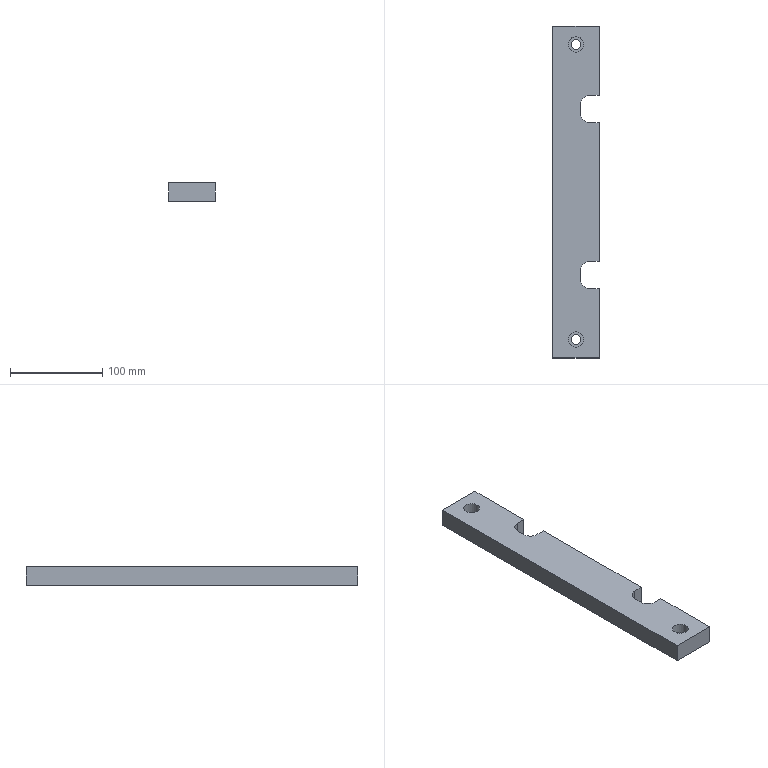Part | STEP file | 200 mesh_id2002 | 1 solid | 24 faces | box 50 x 360 x 20 mm | volume 331105 mm3 | plane 16 | cylinder 8 | commonest cylinder face diameters 20 x4 10.7 x2 17 x2
STEP:
#1=CARTESIAN_POINT('',(-17103.234,-4180.269,185.258));
#2=VERTEX_POINT('',#1);
#3=CARTESIAN_POINT('',(-17097.884,-4180.269,185.258));
#4=DIRECTION('',(0.,0.,1.));
#5=DIRECTION('',(-1.,0.,0.));
#6=AXIS2_PLACEMENT_3D('',#3,#4,#5);
#7=CIRCLE('',#6,5.35);
#8=EDGE_CURVE('',#2,#2,#7,.T.);
#9=ORIENTED_EDGE('',*,*,#8,.F.);
#10=EDGE_LOOP('',(#9));
#11=FACE_BOUND('',#10,.T.);
#12=CARTESIAN_POINT('',(-17106.384,-4180.269,185.258));
#13=VERTEX_POINT('',#12);
#14=CARTESIAN_POINT('',(-17097.884,-4180.269,185.258));
#15=DIRECTION('',(0.,0.,1.));
#16=DIRECTION('',(-1.,0.,0.));
#17=AXIS2_PLACEMENT_3D('',#14,#15,#16);
#18=CIRCLE('',#17,8.5);
#19=EDGE_CURVE('',#13,#13,#18,.T.);
#20=ORIENTED_EDGE('',*,*,#19,.T.);
#21=EDGE_LOOP('',(#20));
#22=FACE_BOUND('',#21,.T.);
#23=CARTESIAN_POINT('',(-17097.884,-4180.269,185.258));
#24=DIRECTION('',(0.,0.,-1.));
#25=DIRECTION('',(-1.,0.,0.));
#26=AXIS2_PLACEMENT_3D('',#23,#24,#25);
#27=PLANE('',#26);
#28=ADVANCED_FACE('',(#11,#22),#27,.F.);
#29=ORIENTED_EDGE('',*,*,#19,.F.);
#30=EDGE_LOOP('',(#29));
#31=FACE_BOUND('',#30,.T.);
#32=CARTESIAN_POINT('',(-17106.384,-4180.269,196.258));
#33=VERTEX_POINT('',#32);
#34=CARTESIAN_POINT('',(-17097.884,-4180.269,196.258));
#35=DIRECTION('',(0.,0.,-1.));
#36=DIRECTION('',(-1.,0.,0.));
#37=AXIS2_PLACEMENT_3D('',#34,#35,#36);
#38=CIRCLE('',#37,8.5);
#39=EDGE_CURVE('',#33,#33,#38,.T.);
#40=ORIENTED_EDGE('',*,*,#39,.F.);
#41=EDGE_LOOP('',(#40));
#42=FACE_BOUND('',#41,.T.);
#43=CARTESIAN_POINT('',(-17097.884,-4180.269,196.258));
#44=DIRECTION('',(0.,0.,-1.));
#45=DIRECTION('',(-1.,0.,0.));
#46=AXIS2_PLACEMENT_3D('',#43,#44,#45);
#47=CYLINDRICAL_SURFACE('',#46,8.5);
#48=ADVANCED_FACE('',(#31,#42),#47,.F.);
#49=ORIENTED_EDGE('',*,*,#8,.T.);
#50=EDGE_LOOP('',(#49));
#51=FACE_BOUND('',#50,.T.);
#52=CARTESIAN_POINT('',(-17092.534,-4180.269,176.258));
#53=VERTEX_POINT('',#52);
#54=CARTESIAN_POINT('',(-17097.884,-4180.269,176.258));
#55=DIRECTION('',(0.,0.,1.));
#56=DIRECTION('',(1.,0.,0.));
#57=AXIS2_PLACEMENT_3D('',#54,#55,#56);
#58=CIRCLE('',#57,5.35);
#59=EDGE_CURVE('',#53,#53,#58,.T.);
#60=ORIENTED_EDGE('',*,*,#59,.F.);
#61=EDGE_LOOP('',(#60));
#62=FACE_BOUND('',#61,.T.);
#63=CARTESIAN_POINT('',(-17097.884,-4180.269,65.92));
#64=DIRECTION('',(0.,0.,-1.));
#65=DIRECTION('',(-1.,0.,0.));
#66=AXIS2_PLACEMENT_3D('',#63,#64,#65);
#67=CYLINDRICAL_SURFACE('',#66,5.35);
#68=ADVANCED_FACE('',(#51,#62),#67,.F.);
#69=CARTESIAN_POINT('',(-17103.234,-3860.269,185.258));
#70=VERTEX_POINT('',#69);
#71=CARTESIAN_POINT('',(-17097.884,-3860.269,185.258));
#72=DIRECTION('',(0.,0.,1.));
#73=DIRECTION('',(-1.,0.,0.));
#74=AXIS2_PLACEMENT_3D('',#71,#72,#73);
#75=CIRCLE('',#74,5.35);
#76=EDGE_CURVE('',#70,#70,#75,.T.);
#77=ORIENTED_EDGE('',*,*,#76,.F.);
#78=EDGE_LOOP('',(#77));
#79=FACE_BOUND('',#78,.T.);
#80=CARTESIAN_POINT('',(-17106.384,-3860.269,185.258));
#81=VERTEX_POINT('',#80);
#82=CARTESIAN_POINT('',(-17097.884,-3860.269,185.258));
#83=DIRECTION('',(0.,0.,1.));
#84=DIRECTION('',(-1.,0.,0.));
#85=AXIS2_PLACEMENT_3D('',#82,#83,#84);
#86=CIRCLE('',#85,8.5);
#87=EDGE_CURVE('',#81,#81,#86,.T.);
#88=ORIENTED_EDGE('',*,*,#87,.T.);
#89=EDGE_LOOP('',(#88));
#90=FACE_BOUND('',#89,.T.);
#91=CARTESIAN_POINT('',(-17097.884,-3860.269,185.258));
#92=DIRECTION('',(0.,0.,-1.));
#93=DIRECTION('',(-1.,0.,0.));
#94=AXIS2_PLACEMENT_3D('',#91,#92,#93);
#95=PLANE('',#94);
#96=ADVANCED_FACE('',(#79,#90),#95,.F.);
#97=CARTESIAN_POINT('',(-17082.884,-3945.269,196.258));
#98=VERTEX_POINT('',#97);
#99=CARTESIAN_POINT('',(-17092.884,-3935.269,196.258));
#100=VERTEX_POINT('',#99);
#101=CARTESIAN_POINT('',(-17082.884,-3935.269,196.258));
#102=DIRECTION('',(0.,0.,-1.));
#103=DIRECTION('',(-1.,0.,0.));
#104=AXIS2_PLACEMENT_3D('',#101,#102,#103);
#105=CIRCLE('',#104,10.);
#106=EDGE_CURVE('',#98,#100,#105,.T.);
#107=ORIENTED_EDGE('',*,*,#106,.F.);
#108=CARTESIAN_POINT('',(-17082.884,-3945.269,176.258));
#109=VERTEX_POINT('',#108);
#110=CARTESIAN_POINT('',(-17082.884,-3945.269,196.258));
#111=DIRECTION('',(0.,0.,1.));
#112=VECTOR('',#111,1.);
#113=LINE('',#110,#112);
#114=EDGE_CURVE('',#109,#98,#113,.T.);
#115=ORIENTED_EDGE('',*,*,#114,.F.);
#116=CARTESIAN_POINT('',(-17092.884,-3935.269,176.258));
#117=VERTEX_POINT('',#116);
#118=CARTESIAN_POINT('',(-17082.884,-3935.269,176.258));
#119=DIRECTION('',(0.,0.,1.));
#120=DIRECTION('',(1.,0.,0.));
#121=AXIS2_PLACEMENT_3D('',#118,#119,#120);
#122=CIRCLE('',#121,10.);
#123=EDGE_CURVE('',#117,#109,#122,.T.);
#124=ORIENTED_EDGE('',*,*,#123,.F.);
#125=CARTESIAN_POINT('',(-17092.884,-3935.269,176.258));
#126=DIRECTION('',(0.,0.,-1.));
#127=VECTOR('',#126,1.);
#128=LINE('',#125,#127);
#129=EDGE_CURVE('',#100,#117,#128,.T.);
#130=ORIENTED_EDGE('',*,*,#129,.F.);
#131=EDGE_LOOP('',(#107,#115,#124,#130));
#132=FACE_OUTER_BOUND('',#131,.T.);
#133=CARTESIAN_POINT('',(-17082.884,-3935.269,176.258));
#134=DIRECTION('',(0.,0.,1.));
#135=DIRECTION('',(1.,0.,0.));
#136=AXIS2_PLACEMENT_3D('',#133,#134,#135);
#137=CYLINDRICAL_SURFACE('',#136,10.);
#138=ADVANCED_FACE('',(#132),#137,.F.);
#139=CARTESIAN_POINT('',(-17072.884,-3945.269,176.258));
#140=VERTEX_POINT('',#139);
#141=CARTESIAN_POINT('',(-17082.884,-3945.269,176.258));
#142=DIRECTION('',(1.,0.,0.));
#143=VECTOR('',#142,1.);
#144=LINE('',#141,#143);
#145=EDGE_CURVE('',#109,#140,#144,.T.);
#146=ORIENTED_EDGE('',*,*,#145,.F.);
#147=ORIENTED_EDGE('',*,*,#114,.T.);
#148=CARTESIAN_POINT('',(-17072.884,-3945.269,196.258));
#149=VERTEX_POINT('',#148);
#150=CARTESIAN_POINT('',(-17082.884,-3945.269,196.258));
#151=DIRECTION('',(-1.,0.,0.));
#152=VECTOR('',#151,1.);
#153=LINE('',#150,#152);
#154=EDGE_CURVE('',#149,#98,#153,.T.);
#155=ORIENTED_EDGE('',*,*,#154,.F.);
#156=CARTESIAN_POINT('',(-17072.884,-3945.269,176.258));
#157=DIRECTION('',(0.,0.,1.));
#158=VECTOR('',#157,1.);
#159=LINE('',#156,#158);
#160=EDGE_CURVE('',#140,#149,#159,.T.);
#161=ORIENTED_EDGE('',*,*,#160,.F.);
#162=EDGE_LOOP('',(#146,#147,#155,#161));
#163=FACE_OUTER_BOUND('',#162,.T.);
#164=CARTESIAN_POINT('',(-17082.884,-3945.269,176.258));
#165=DIRECTION('',(0.,-1.,0.));
#166=DIRECTION('',(0.,0.,-1.));
#167=AXIS2_PLACEMENT_3D('',#164,#165,#166);
#168=PLANE('',#167);
#169=ADVANCED_FACE('',(#163),#168,.F.);
#170=CARTESIAN_POINT('',(-17072.884,-4095.269,176.258));
#171=VERTEX_POINT('',#170);
#172=CARTESIAN_POINT('',(-17072.884,-3830.269,176.258));
#173=DIRECTION('',(0.,-1.,0.));
#174=VECTOR('',#173,1.);
#175=LINE('',#172,#174);
#176=EDGE_CURVE('',#140,#171,#175,.T.);
#177=ORIENTED_EDGE('',*,*,#176,.F.);
#178=ORIENTED_EDGE('',*,*,#160,.T.);
#179=CARTESIAN_POINT('',(-17072.884,-4095.269,196.258));
#180=VERTEX_POINT('',#179);
#181=CARTESIAN_POINT('',(-17072.884,-4210.269,196.258));
#182=DIRECTION('',(0.,1.,0.));
#183=VECTOR('',#182,1.);
#184=LINE('',#181,#183);
#185=EDGE_CURVE('',#180,#149,#184,.T.);
#186=ORIENTED_EDGE('',*,*,#185,.F.);
#187=CARTESIAN_POINT('',(-17072.884,-4095.269,176.258));
#188=DIRECTION('',(0.,0.,1.));
#189=VECTOR('',#188,1.);
#190=LINE('',#187,#189);
#191=EDGE_CURVE('',#171,#180,#190,.T.);
#192=ORIENTED_EDGE('',*,*,#191,.F.);
#193=EDGE_LOOP('',(#177,#178,#186,#192));
#194=FACE_OUTER_BOUND('',#193,.T.);
#195=CARTESIAN_POINT('',(-17072.884,0.,15.));
#196=DIRECTION('',(-1.,0.,0.));
#197=DIRECTION('',(0.,0.,1.));
#198=AXIS2_PLACEMENT_3D('',#195,#196,#197);
#199=PLANE('',#198);
#200=ADVANCED_FACE('',(#194),#199,.F.);
#201=CARTESIAN_POINT('',(-17082.884,-4095.269,196.258));
#202=VERTEX_POINT('',#201);
#203=CARTESIAN_POINT('',(-17082.884,-4095.269,196.258));
#204=DIRECTION('',(1.,0.,0.));
#205=VECTOR('',#204,1.);
#206=LINE('',#203,#205);
#207=EDGE_CURVE('',#202,#180,#206,.T.);
#208=ORIENTED_EDGE('',*,*,#207,.F.);
#209=CARTESIAN_POINT('',(-17082.884,-4095.269,176.258));
#210=VERTEX_POINT('',#209);
#211=CARTESIAN_POINT('',(-17082.884,-4095.269,176.258));
#212=DIRECTION('',(0.,0.,-1.));
#213=VECTOR('',#212,1.);
#214=LINE('',#211,#213);
#215=EDGE_CURVE('',#202,#210,#214,.T.);
#216=ORIENTED_EDGE('',*,*,#215,.T.);
#217=CARTESIAN_POINT('',(-17082.884,-4095.269,176.258));
#218=DIRECTION('',(-1.,0.,0.));
#219=VECTOR('',#218,1.);
#220=LINE('',#217,#219);
#221=EDGE_CURVE('',#171,#210,#220,.T.);
#222=ORIENTED_EDGE('',*,*,#221,.F.);
#223=ORIENTED_EDGE('',*,*,#191,.T.);
#224=EDGE_LOOP('',(#208,#216,#222,#223));
#225=FACE_OUTER_BOUND('',#224,.T.);
#226=CARTESIAN_POINT('',(-17082.884,-4095.269,176.258));
#227=DIRECTION('',(0.,1.,0.));
#228=DIRECTION('',(0.,0.,1.));
#229=AXIS2_PLACEMENT_3D('',#226,#227,#228);
#230=PLANE('',#229);
#231=ADVANCED_FACE('',(#225),#230,.F.);
#232=CARTESIAN_POINT('',(-17092.884,-4105.269,196.258));
#233=VERTEX_POINT('',#232);
#234=CARTESIAN_POINT('',(-17082.884,-4105.269,196.258));
#235=DIRECTION('',(0.,0.,-1.));
#236=DIRECTION('',(-1.,0.,0.));
#237=AXIS2_PLACEMENT_3D('',#234,#235,#236);
#238=CIRCLE('',#237,10.);
#239=EDGE_CURVE('',#233,#202,#238,.T.);
#240=ORIENTED_EDGE('',*,*,#239,.F.);
#241=CARTESIAN_POINT('',(-17092.884,-4105.269,176.258));
#242=VERTEX_POINT('',#241);
#243=CARTESIAN_POINT('',(-17092.884,-4105.269,196.258));
#244=DIRECTION('',(0.,0.,1.));
#245=VECTOR('',#244,1.);
#246=LINE('',#243,#245);
#247=EDGE_CURVE('',#242,#233,#246,.T.);
#248=ORIENTED_EDGE('',*,*,#247,.F.);
#249=CARTESIAN_POINT('',(-17082.884,-4105.269,176.258));
#250=DIRECTION('',(0.,0.,1.));
#251=DIRECTION('',(1.,0.,0.));
#252=AXIS2_PLACEMENT_3D('',#249,#250,#251);
#253=CIRCLE('',#252,10.);
#254=EDGE_CURVE('',#210,#242,#253,.T.);
#255=ORIENTED_EDGE('',*,*,#254,.F.);
#256=ORIENTED_EDGE('',*,*,#215,.F.);
#257=EDGE_LOOP('',(#240,#248,#255,#256));
#258=FACE_OUTER_BOUND('',#257,.T.);
#259=CARTESIAN_POINT('',(-17082.884,-4105.269,176.258));
#260=DIRECTION('',(0.,0.,1.));
#261=DIRECTION('',(1.,0.,0.));
#262=AXIS2_PLACEMENT_3D('',#259,#260,#261);
#263=CYLINDRICAL_SURFACE('',#262,10.);
#264=ADVANCED_FACE('',(#258),#263,.F.);
#265=CARTESIAN_POINT('',(-17092.884,-4115.269,196.258));
#266=VERTEX_POINT('',#265);
#267=CARTESIAN_POINT('',(-17092.884,-4110.269,196.258));
#268=DIRECTION('',(0.,1.,0.));
#269=VECTOR('',#268,1.);
#270=LINE('',#267,#269);
#271=EDGE_CURVE('',#266,#233,#270,.T.);
#272=ORIENTED_EDGE('',*,*,#271,.F.);
#273=CARTESIAN_POINT('',(-17092.884,-4115.269,176.258));
#274=VERTEX_POINT('',#273);
#275=CARTESIAN_POINT('',(-17092.884,-4115.269,176.258));
#276=DIRECTION('',(0.,0.,-1.));
#277=VECTOR('',#276,1.);
#278=LINE('',#275,#277);
#279=EDGE_CURVE('',#266,#274,#278,.T.);
#280=ORIENTED_EDGE('',*,*,#279,.T.);
#281=CARTESIAN_POINT('',(-17092.884,-4110.269,176.258));
#282=DIRECTION('',(0.,-1.,0.));
#283=VECTOR('',#282,1.);
#284=LINE('',#281,#283);
#285=EDGE_CURVE('',#242,#274,#284,.T.);
#286=ORIENTED_EDGE('',*,*,#285,.F.);
#287=ORIENTED_EDGE('',*,*,#247,.T.);
#288=EDGE_LOOP('',(#272,#280,#286,#287));
#289=FACE_OUTER_BOUND('',#288,.T.);
#290=CARTESIAN_POINT('',(-17092.884,-4110.269,176.258));
#291=DIRECTION('',(-1.,0.,0.));
#292=DIRECTION('',(0.,0.,1.));
#293=AXIS2_PLACEMENT_3D('',#290,#291,#292);
#294=PLANE('',#293);
#295=ADVANCED_FACE('',(#289),#294,.F.);
#296=CARTESIAN_POINT('',(-17082.884,-4125.269,196.258));
#297=VERTEX_POINT('',#296);
#298=CARTESIAN_POINT('',(-17082.884,-4115.269,196.258));
#299=DIRECTION('',(0.,0.,-1.));
#300=DIRECTION('',(-1.,0.,0.));
#301=AXIS2_PLACEMENT_3D('',#298,#299,#300);
#302=CIRCLE('',#301,10.);
#303=EDGE_CURVE('',#297,#266,#302,.T.);
#304=ORIENTED_EDGE('',*,*,#303,.F.);
#305=CARTESIAN_POINT('',(-17082.884,-4125.269,176.258));
#306=VERTEX_POINT('',#305);
#307=CARTESIAN_POINT('',(-17082.884,-4125.269,196.258));
#308=DIRECTION('',(0.,0.,1.));
#309=VECTOR('',#308,1.);
#310=LINE('',#307,#309);
#311=EDGE_CURVE('',#306,#297,#310,.T.);
#312=ORIENTED_EDGE('',*,*,#311,.F.);
#313=CARTESIAN_POINT('',(-17082.884,-4115.269,176.258));
#314=DIRECTION('',(0.,0.,1.));
#315=DIRECTION('',(1.,0.,0.));
#316=AXIS2_PLACEMENT_3D('',#313,#314,#315);
#317=CIRCLE('',#316,10.);
#318=EDGE_CURVE('',#274,#306,#317,.T.);
#319=ORIENTED_EDGE('',*,*,#318,.F.);
#320=ORIENTED_EDGE('',*,*,#279,.F.);
#321=EDGE_LOOP('',(#304,#312,#319,#320));
#322=FACE_OUTER_BOUND('',#321,.T.);
#323=CARTESIAN_POINT('',(-17082.884,-4115.269,176.258));
#324=DIRECTION('',(0.,0.,1.));
#325=DIRECTION('',(1.,0.,0.));
#326=AXIS2_PLACEMENT_3D('',#323,#324,#325);
#327=CYLINDRICAL_SURFACE('',#326,10.);
#328=ADVANCED_FACE('',(#322),#327,.F.);
#329=CARTESIAN_POINT('',(-17072.884,-4125.269,176.258));
#330=VERTEX_POINT('',#329);
#331=CARTESIAN_POINT('',(-17082.884,-4125.269,176.258));
#332=DIRECTION('',(1.,0.,0.));
#333=VECTOR('',#332,1.);
#334=LINE('',#331,#333);
#335=EDGE_CURVE('',#306,#330,#334,.T.);
#336=ORIENTED_EDGE('',*,*,#335,.F.);
#337=ORIENTED_EDGE('',*,*,#311,.T.);
#338=CARTESIAN_POINT('',(-17072.884,-4125.269,196.258));
#339=VERTEX_POINT('',#338);
#340=CARTESIAN_POINT('',(-17082.884,-4125.269,196.258));
#341=DIRECTION('',(-1.,0.,0.));
#342=VECTOR('',#341,1.);
#343=LINE('',#340,#342);
#344=EDGE_CURVE('',#339,#297,#343,.T.);
#345=ORIENTED_EDGE('',*,*,#344,.F.);
#346=CARTESIAN_POINT('',(-17072.884,-4125.269,176.258));
#347=DIRECTION('',(0.,0.,1.));
#348=VECTOR('',#347,1.);
#349=LINE('',#346,#348);
#350=EDGE_CURVE('',#330,#339,#349,.T.);
#351=ORIENTED_EDGE('',*,*,#350,.F.);
#352=EDGE_LOOP('',(#336,#337,#345,#351));
#353=FACE_OUTER_BOUND('',#352,.T.);
#354=CARTESIAN_POINT('',(-17082.884,-4125.269,176.258));
#355=DIRECTION('',(0.,-1.,0.));
#356=DIRECTION('',(0.,0.,-1.));
#357=AXIS2_PLACEMENT_3D('',#354,#355,#356);
#358=PLANE('',#357);
#359=ADVANCED_FACE('',(#353),#358,.F.);
#360=CARTESIAN_POINT('',(-17072.884,-4200.269,176.258));
#361=VERTEX_POINT('',#360);
#362=CARTESIAN_POINT('',(-17072.884,-3830.269,176.258));
#363=DIRECTION('',(0.,-1.,0.));
#364=VECTOR('',#363,1.);
#365=LINE('',#362,#364);
#366=EDGE_CURVE('',#330,#361,#365,.T.);
#367=ORIENTED_EDGE('',*,*,#366,.F.);
#368=ORIENTED_EDGE('',*,*,#350,.T.);
#369=CARTESIAN_POINT('',(-17072.884,-4200.269,196.258));
#370=VERTEX_POINT('',#369);
#371=CARTESIAN_POINT('',(-17072.884,-4210.269,196.258));
#372=DIRECTION('',(0.,1.,0.));
#373=VECTOR('',#372,1.);
#374=LINE('',#371,#373);
#375=EDGE_CURVE('',#370,#339,#374,.T.);
#376=ORIENTED_EDGE('',*,*,#375,.F.);
#377=CARTESIAN_POINT('',(-17072.884,-4200.269,176.258));
#378=DIRECTION('',(0.,0.,1.));
#379=VECTOR('',#378,1.);
#380=LINE('',#377,#379);
#381=EDGE_CURVE('',#361,#370,#380,.T.);
#382=ORIENTED_EDGE('',*,*,#381,.F.);
#383=EDGE_LOOP('',(#367,#368,#376,#382));
#384=FACE_OUTER_BOUND('',#383,.T.);
#385=CARTESIAN_POINT('',(-17072.884,0.,15.));
#386=DIRECTION('',(-1.,0.,0.));
#387=DIRECTION('',(0.,0.,1.));
#388=AXIS2_PLACEMENT_3D('',#385,#386,#387);
#389=PLANE('',#388);
#390=ADVANCED_FACE('',(#384),#389,.F.);
#391=ORIENTED_EDGE('',*,*,#381,.T.);
#392=CARTESIAN_POINT('',(-17122.884,-4200.269,196.258));
#393=VERTEX_POINT('',#392);
#394=CARTESIAN_POINT('',(-17132.884,-4200.269,196.258));
#395=DIRECTION('',(1.,0.,0.));
#396=VECTOR('',#395,1.);
#397=LINE('',#394,#396);
#398=EDGE_CURVE('',#393,#370,#397,.T.);
#399=ORIENTED_EDGE('',*,*,#398,.F.);
#400=CARTESIAN_POINT('',(-17122.884,-4200.269,176.258));
#401=VERTEX_POINT('',#400);
#402=CARTESIAN_POINT('',(-17122.884,-4200.269,176.258));
#403=DIRECTION('',(0.,0.,1.));
#404=VECTOR('',#403,1.);
#405=LINE('',#402,#404);
#406=EDGE_CURVE('',#401,#393,#405,.T.);
#407=ORIENTED_EDGE('',*,*,#406,.F.);
#408=CARTESIAN_POINT('',(-17132.884,-4200.269,176.258));
#409=DIRECTION('',(1.,0.,0.));
#410=VECTOR('',#409,1.);
#411=LINE('',#408,#410);
#412=EDGE_CURVE('',#401,#361,#411,.T.);
#413=ORIENTED_EDGE('',*,*,#412,.T.);
#414=EDGE_LOOP('',(#391,#399,#407,#413));
#415=FACE_OUTER_BOUND('',#414,.T.);
#416=CARTESIAN_POINT('',(-17132.884,-4200.269,176.258));
#417=DIRECTION('',(0.,1.,0.));
#418=DIRECTION('',(0.,0.,1.));
#419=AXIS2_PLACEMENT_3D('',#416,#417,#418);
#420=PLANE('',#419);
#421=ADVANCED_FACE('',(#415),#420,.F.);
#422=ORIENTED_EDGE('',*,*,#406,.T.);
#423=CARTESIAN_POINT('',(-17122.884,-3840.269,196.258));
#424=VERTEX_POINT('',#423);
#425=CARTESIAN_POINT('',(-17122.884,-4210.269,196.258));
#426=DIRECTION('',(0.,1.,0.));
#427=VECTOR('',#426,1.);
#428=LINE('',#425,#427);
#429=EDGE_CURVE('',#393,#424,#428,.T.);
#430=ORIENTED_EDGE('',*,*,#429,.T.);
#431=CARTESIAN_POINT('',(-17122.884,-3840.269,176.258));
#432=VERTEX_POINT('',#431);
#433=CARTESIAN_POINT('',(-17122.884,-3840.269,196.258));
#434=DIRECTION('',(0.,0.,-1.));
#435=VECTOR('',#434,1.);
#436=LINE('',#433,#435);
#437=EDGE_CURVE('',#424,#432,#436,.T.);
#438=ORIENTED_EDGE('',*,*,#437,.T.);
#439=CARTESIAN_POINT('',(-17122.884,-3830.269,176.258));
#440=DIRECTION('',(0.,-1.,0.));
#441=VECTOR('',#440,1.);
#442=LINE('',#439,#441);
#443=EDGE_CURVE('',#432,#401,#442,.T.);
#444=ORIENTED_EDGE('',*,*,#443,.T.);
#445=EDGE_LOOP('',(#422,#430,#438,#444));
#446=FACE_OUTER_BOUND('',#445,.T.);
#447=CARTESIAN_POINT('',(-17122.884,-4180.269,126.258));
#448=DIRECTION('',(1.,0.,0.));
#449=DIRECTION('',(0.,0.,-1.));
#450=AXIS2_PLACEMENT_3D('',#447,#448,#449);
#451=PLANE('',#450);
#452=ADVANCED_FACE('',(#446),#451,.F.);
#453=CARTESIAN_POINT('',(-17072.884,-3840.269,196.258));
#454=VERTEX_POINT('',#453);
#455=CARTESIAN_POINT('',(-17072.884,-3840.269,176.258));
#456=VERTEX_POINT('',#455);
#457=CARTESIAN_POINT('',(-17072.884,-3840.269,196.258));
#458=DIRECTION('',(0.,0.,-1.));
#459=VECTOR('',#458,1.);
#460=LINE('',#457,#459);
#461=EDGE_CURVE('',#454,#456,#460,.T.);
#462=ORIENTED_EDGE('',*,*,#461,.T.);
#463=CARTESIAN_POINT('',(-17132.884,-3840.269,176.258));
#464=DIRECTION('',(1.,0.,0.));
#465=VECTOR('',#464,1.);
#466=LINE('',#463,#465);
#467=EDGE_CURVE('',#432,#456,#466,.T.);
#468=ORIENTED_EDGE('',*,*,#467,.F.);
#469=ORIENTED_EDGE('',*,*,#437,.F.);
#470=CARTESIAN_POINT('',(-17132.884,-3840.269,196.258));
#471=DIRECTION('',(1.,0.,0.));
#472=VECTOR('',#471,1.);
#473=LINE('',#470,#472);
#474=EDGE_CURVE('',#424,#454,#473,.T.);
#475=ORIENTED_EDGE('',*,*,#474,.T.);
#476=EDGE_LOOP('',(#462,#468,#469,#475));
#477=FACE_OUTER_BOUND('',#476,.T.);
#478=CARTESIAN_POINT('',(-17132.884,-3840.269,196.258));
#479=DIRECTION('',(0.,-1.,0.));
#480=DIRECTION('',(0.,0.,-1.));
#481=AXIS2_PLACEMENT_3D('',#478,#479,#480);
#482=PLANE('',#481);
#483=ADVANCED_FACE('',(#477),#482,.F.);
#484=CARTESIAN_POINT('',(-17072.884,-3915.269,176.258));
#485=VERTEX_POINT('',#484);
#486=CARTESIAN_POINT('',(-17072.884,-3915.269,196.258));
#487=VERTEX_POINT('',#486);
#488=CARTESIAN_POINT('',(-17072.884,-3915.269,176.258));
#489=DIRECTION('',(0.,0.,1.));
#490=VECTOR('',#489,1.);
#491=LINE('',#488,#490);
#492=EDGE_CURVE('',#485,#487,#491,.T.);
#493=ORIENTED_EDGE('',*,*,#492,.F.);
#494=CARTESIAN_POINT('',(-17072.884,-3830.269,176.258));
#495=DIRECTION('',(0.,-1.,0.));
#496=VECTOR('',#495,1.);
#497=LINE('',#494,#496);
#498=EDGE_CURVE('',#456,#485,#497,.T.);
#499=ORIENTED_EDGE('',*,*,#498,.F.);
#500=ORIENTED_EDGE('',*,*,#461,.F.);
#501=CARTESIAN_POINT('',(-17072.884,-4210.269,196.258));
#502=DIRECTION('',(0.,1.,0.));
#503=VECTOR('',#502,1.);
#504=LINE('',#501,#503);
#505=EDGE_CURVE('',#487,#454,#504,.T.);
#506=ORIENTED_EDGE('',*,*,#505,.F.);
#507=EDGE_LOOP('',(#493,#499,#500,#506));
#508=FACE_OUTER_BOUND('',#507,.T.);
#509=CARTESIAN_POINT('',(-17072.884,0.,15.));
#510=DIRECTION('',(-1.,0.,0.));
#511=DIRECTION('',(0.,0.,1.));
#512=AXIS2_PLACEMENT_3D('',#509,#510,#511);
#513=PLANE('',#512);
#514=ADVANCED_FACE('',(#508),#513,.F.);
#515=CARTESIAN_POINT('',(-17082.884,-3915.269,196.258));
#516=VERTEX_POINT('',#515);
#517=CARTESIAN_POINT('',(-17082.884,-3915.269,196.258));
#518=DIRECTION('',(1.,0.,0.));
#519=VECTOR('',#518,1.);
#520=LINE('',#517,#519);
#521=EDGE_CURVE('',#516,#487,#520,.T.);
#522=ORIENTED_EDGE('',*,*,#521,.F.);
#523=CARTESIAN_POINT('',(-17082.884,-3915.269,176.258));
#524=VERTEX_POINT('',#523);
#525=CARTESIAN_POINT('',(-17082.884,-3915.269,176.258));
#526=DIRECTION('',(0.,0.,-1.));
#527=VECTOR('',#526,1.);
#528=LINE('',#525,#527);
#529=EDGE_CURVE('',#516,#524,#528,.T.);
#530=ORIENTED_EDGE('',*,*,#529,.T.);
#531=CARTESIAN_POINT('',(-17082.884,-3915.269,176.258));
#532=DIRECTION('',(-1.,0.,0.));
#533=VECTOR('',#532,1.);
#534=LINE('',#531,#533);
#535=EDGE_CURVE('',#485,#524,#534,.T.);
#536=ORIENTED_EDGE('',*,*,#535,.F.);
#537=ORIENTED_EDGE('',*,*,#492,.T.);
#538=EDGE_LOOP('',(#522,#530,#536,#537));
#539=FACE_OUTER_BOUND('',#538,.T.);
#540=CARTESIAN_POINT('',(-17082.884,-3915.269,176.258));
#541=DIRECTION('',(0.,1.,0.));
#542=DIRECTION('',(0.,0.,1.));
#543=AXIS2_PLACEMENT_3D('',#540,#541,#542);
#544=PLANE('',#543);
#545=ADVANCED_FACE('',(#539),#544,.F.);
#546=CARTESIAN_POINT('',(-17092.884,-3925.269,196.258));
#547=VERTEX_POINT('',#546);
#548=CARTESIAN_POINT('',(-17082.884,-3925.269,196.258));
#549=DIRECTION('',(0.,0.,-1.));
#550=DIRECTION('',(-1.,0.,0.));
#551=AXIS2_PLACEMENT_3D('',#548,#549,#550);
#552=CIRCLE('',#551,10.);
#553=EDGE_CURVE('',#547,#516,#552,.T.);
#554=ORIENTED_EDGE('',*,*,#553,.F.);
#555=CARTESIAN_POINT('',(-17092.884,-3925.269,176.258));
#556=VERTEX_POINT('',#555);
#557=CARTESIAN_POINT('',(-17092.884,-3925.269,196.258));
#558=DIRECTION('',(0.,0.,1.));
#559=VECTOR('',#558,1.);
#560=LINE('',#557,#559);
#561=EDGE_CURVE('',#556,#547,#560,.T.);
#562=ORIENTED_EDGE('',*,*,#561,.F.);
#563=CARTESIAN_POINT('',(-17082.884,-3925.269,176.258));
#564=DIRECTION('',(0.,0.,1.));
#565=DIRECTION('',(1.,0.,0.));
#566=AXIS2_PLACEMENT_3D('',#563,#564,#565);
#567=CIRCLE('',#566,10.);
#568=EDGE_CURVE('',#524,#556,#567,.T.);
#569=ORIENTED_EDGE('',*,*,#568,.F.);
#570=ORIENTED_EDGE('',*,*,#529,.F.);
#571=EDGE_LOOP('',(#554,#562,#569,#570));
#572=FACE_OUTER_BOUND('',#571,.T.);
#573=CARTESIAN_POINT('',(-17082.884,-3925.269,176.258));
#574=DIRECTION('',(0.,0.,1.));
#575=DIRECTION('',(1.,0.,0.));
#576=AXIS2_PLACEMENT_3D('',#573,#574,#575);
#577=CYLINDRICAL_SURFACE('',#576,10.);
#578=ADVANCED_FACE('',(#572),#577,.F.);
#579=CARTESIAN_POINT('',(-17092.884,-3930.269,176.258));
#580=DIRECTION('',(0.,-1.,0.));
#581=VECTOR('',#580,1.);
#582=LINE('',#579,#581);
#583=EDGE_CURVE('',#556,#117,#582,.T.);
#584=ORIENTED_EDGE('',*,*,#583,.F.);
#585=ORIENTED_EDGE('',*,*,#561,.T.);
#586=CARTESIAN_POINT('',(-17092.884,-3930.269,196.258));
#587=DIRECTION('',(0.,1.,0.));
#588=VECTOR('',#587,1.);
#589=LINE('',#586,#588);
#590=EDGE_CURVE('',#100,#547,#589,.T.);
#591=ORIENTED_EDGE('',*,*,#590,.F.);
#592=ORIENTED_EDGE('',*,*,#129,.T.);
#593=EDGE_LOOP('',(#584,#585,#591,#592));
#594=FACE_OUTER_BOUND('',#593,.T.);
#595=CARTESIAN_POINT('',(-17092.884,-3930.269,176.258));
#596=DIRECTION('',(-1.,0.,0.));
#597=DIRECTION('',(0.,0.,1.));
#598=AXIS2_PLACEMENT_3D('',#595,#596,#597);
#599=PLANE('',#598);
#600=ADVANCED_FACE('',(#594),#599,.F.);
#601=ORIENTED_EDGE('',*,*,#87,.F.);
#602=EDGE_LOOP('',(#601));
#603=FACE_BOUND('',#602,.T.);
#604=CARTESIAN_POINT('',(-17106.384,-3860.269,196.258));
#605=VERTEX_POINT('',#604);
#606=CARTESIAN_POINT('',(-17097.884,-3860.269,196.258));
#607=DIRECTION('',(0.,0.,-1.));
#608=DIRECTION('',(-1.,0.,0.));
#609=AXIS2_PLACEMENT_3D('',#606,#607,#608);
#610=CIRCLE('',#609,8.5);
#611=EDGE_CURVE('',#605,#605,#610,.T.);
#612=ORIENTED_EDGE('',*,*,#611,.F.);
#613=EDGE_LOOP('',(#612));
#614=FACE_BOUND('',#613,.T.);
#615=CARTESIAN_POINT('',(-17097.884,-3860.269,196.258));
#616=DIRECTION('',(0.,0.,-1.));
#617=DIRECTION('',(-1.,0.,0.));
#618=AXIS2_PLACEMENT_3D('',#615,#616,#617);
#619=CYLINDRICAL_SURFACE('',#618,8.5);
#620=ADVANCED_FACE('',(#603,#614),#619,.F.);
#621=ORIENTED_EDGE('',*,*,#39,.T.);
#622=EDGE_LOOP('',(#621));
#623=FACE_BOUND('',#622,.T.);
#624=ORIENTED_EDGE('',*,*,#611,.T.);
#625=EDGE_LOOP('',(#624));
#626=FACE_BOUND('',#625,.T.);
#627=ORIENTED_EDGE('',*,*,#590,.T.);
#628=ORIENTED_EDGE('',*,*,#553,.T.);
#629=ORIENTED_EDGE('',*,*,#521,.T.);
#630=ORIENTED_EDGE('',*,*,#505,.T.);
#631=ORIENTED_EDGE('',*,*,#474,.F.);
#632=ORIENTED_EDGE('',*,*,#429,.F.);
#633=ORIENTED_EDGE('',*,*,#398,.T.);
#634=ORIENTED_EDGE('',*,*,#375,.T.);
#635=ORIENTED_EDGE('',*,*,#344,.T.);
#636=ORIENTED_EDGE('',*,*,#303,.T.);
#637=ORIENTED_EDGE('',*,*,#271,.T.);
#638=ORIENTED_EDGE('',*,*,#239,.T.);
#639=ORIENTED_EDGE('',*,*,#207,.T.);
#640=ORIENTED_EDGE('',*,*,#185,.T.);
#641=ORIENTED_EDGE('',*,*,#154,.T.);
#642=ORIENTED_EDGE('',*,*,#106,.T.);
#643=EDGE_LOOP('',(#627,#628,#629,#630,#631,#632,#633,#634,#635,#636,#637,#638,#639,#640,#641,#642));
#644=FACE_BOUND('',#643,.T.);
#645=CARTESIAN_POINT('',(-17132.884,-4210.269,196.258));
#646=DIRECTION('',(0.,0.,-1.));
#647=DIRECTION('',(-1.,0.,0.));
#648=AXIS2_PLACEMENT_3D('',#645,#646,#647);
#649=PLANE('',#648);
#650=ADVANCED_FACE('',(#623,#626,#644),#649,.F.);
#651=ORIENTED_EDGE('',*,*,#76,.T.);
#652=EDGE_LOOP('',(#651));
#653=FACE_BOUND('',#652,.T.);
#654=CARTESIAN_POINT('',(-17092.534,-3860.269,176.258));
#655=VERTEX_POINT('',#654);
#656=CARTESIAN_POINT('',(-17097.884,-3860.269,176.258));
#657=DIRECTION('',(0.,0.,1.));
#658=DIRECTION('',(1.,0.,0.));
#659=AXIS2_PLACEMENT_3D('',#656,#657,#658);
#660=CIRCLE('',#659,5.35);
#661=EDGE_CURVE('',#655,#655,#660,.T.);
#662=ORIENTED_EDGE('',*,*,#661,.F.);
#663=EDGE_LOOP('',(#662));
#664=FACE_BOUND('',#663,.T.);
#665=CARTESIAN_POINT('',(-17097.884,-3860.269,65.92));
#666=DIRECTION('',(0.,0.,-1.));
#667=DIRECTION('',(-1.,0.,0.));
#668=AXIS2_PLACEMENT_3D('',#665,#666,#667);
#669=CYLINDRICAL_SURFACE('',#668,5.35);
#670=ADVANCED_FACE('',(#653,#664),#669,.F.);
#671=ORIENTED_EDGE('',*,*,#59,.T.);
#672=EDGE_LOOP('',(#671));
#673=FACE_BOUND('',#672,.T.);
#674=ORIENTED_EDGE('',*,*,#661,.T.);
#675=EDGE_LOOP('',(#674));
#676=FACE_BOUND('',#675,.T.);
#677=ORIENTED_EDGE('',*,*,#535,.T.);
#678=ORIENTED_EDGE('',*,*,#568,.T.);
#679=ORIENTED_EDGE('',*,*,#583,.T.);
#680=ORIENTED_EDGE('',*,*,#123,.T.);
#681=ORIENTED_EDGE('',*,*,#145,.T.);
#682=ORIENTED_EDGE('',*,*,#176,.T.);
#683=ORIENTED_EDGE('',*,*,#221,.T.);
#684=ORIENTED_EDGE('',*,*,#254,.T.);
#685=ORIENTED_EDGE('',*,*,#285,.T.);
#686=ORIENTED_EDGE('',*,*,#318,.T.);
#687=ORIENTED_EDGE('',*,*,#335,.T.);
#688=ORIENTED_EDGE('',*,*,#366,.T.);
#689=ORIENTED_EDGE('',*,*,#412,.F.);
#690=ORIENTED_EDGE('',*,*,#443,.F.);
#691=ORIENTED_EDGE('',*,*,#467,.T.);
#692=ORIENTED_EDGE('',*,*,#498,.T.);
#693=EDGE_LOOP('',(#677,#678,#679,#680,#681,#682,#683,#684,#685,#686,#687,#688,#689,#690,#691,#692));
#694=FACE_BOUND('',#693,.T.);
#695=CARTESIAN_POINT('',(-17132.884,-3830.269,176.258));
#696=DIRECTION('',(0.,0.,1.));
#697=DIRECTION('',(1.,0.,0.));
#698=AXIS2_PLACEMENT_3D('',#695,#696,#697);
#699=PLANE('',#698);
#700=ADVANCED_FACE('',(#673,#676,#694),#699,.F.);
#701=CLOSED_SHELL('',(#28,#48,#68,#96,#138,#169,#200,#231,#264,#295,#328,#359,#390,#421,#452,#483,#514,#545,#578,#600,#620,#650,#670,#700));
#702=MANIFOLD_SOLID_BREP('',#701);
#703=(LENGTH_UNIT()NAMED_UNIT(*)SI_UNIT(.MILLI.,.METRE.));
#704=UNCERTAINTY_MEASURE_WITH_UNIT(LENGTH_MEASURE(0.00002),#703,'','');
#705=(NAMED_UNIT(*)PLANE_ANGLE_UNIT()SI_UNIT($,.RADIAN.));
#706=PLANE_ANGLE_MEASURE_WITH_UNIT(PLANE_ANGLE_MEASURE(0.01745),#705);
#707=DIMENSIONAL_EXPONENTS(0.,0.,0.,0.,0.,0.,0.);
#708=(CONVERSION_BASED_UNIT('DEGREE',#706)NAMED_UNIT(#707)PLANE_ANGLE_UNIT());
#709=(NAMED_UNIT(*)SI_UNIT($,.STERADIAN.)SOLID_ANGLE_UNIT());
#710=(GEOMETRIC_REPRESENTATION_CONTEXT(3)GLOBAL_UNCERTAINTY_ASSIGNED_CONTEXT((#704))GLOBAL_UNIT_ASSIGNED_CONTEXT((#703,#708,#709))REPRESENTATION_CONTEXT('',''));
#711=ADVANCED_BREP_SHAPE_REPRESENTATION('',(#702),#710);